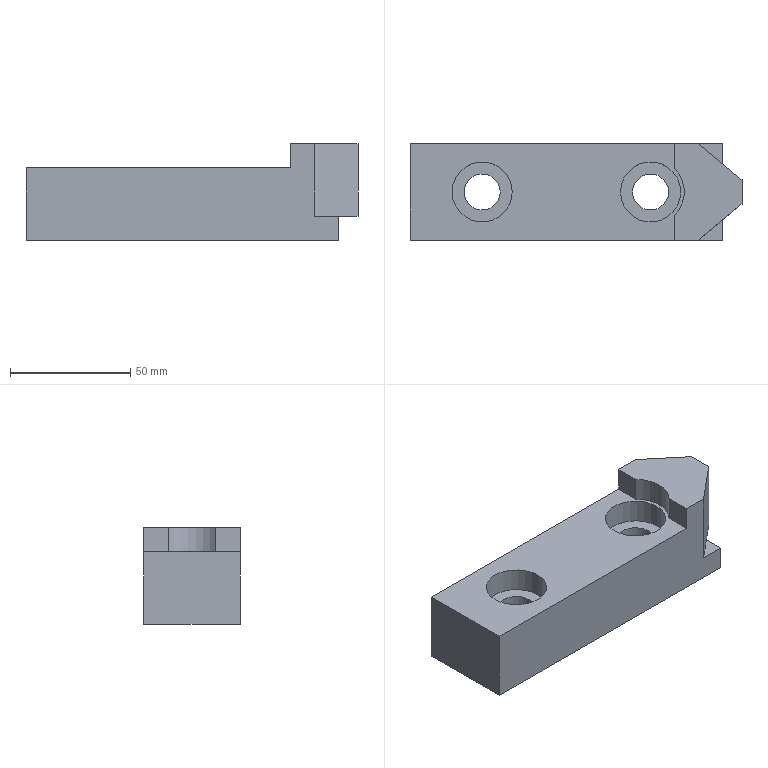Part | SolidWorks | features ICE 5, Extrusion 1 | 1 solid | 26 faces | box 138 x 40 x 40 mm | volume 148074 mm3 | plane 17 | cylinder 9 | commonest cylinder face diameters 15 x4 25 x4 28 x1
STEP:
#1=CARTESIAN_POINT('',(-47.5,0.,20.));
#2=VERTEX_POINT('',#1);
#3=CARTESIAN_POINT('',(-22.5,0.,20.));
#4=VERTEX_POINT('',#3);
#5=CARTESIAN_POINT('',(-35.,0.,20.));
#6=DIRECTION('',(0.,0.,1.));
#7=DIRECTION('',(1.,0.,0.));
#8=AXIS2_PLACEMENT_3D('',#5,#6,#7);
#9=CIRCLE('',#8,12.5);
#10=EDGE_CURVE('',#2,#4,#9,.T.);
#11=ORIENTED_EDGE('',*,*,#10,.F.);
#12=CARTESIAN_POINT('',(-47.5,0.,30.));
#13=VERTEX_POINT('',#12);
#14=CARTESIAN_POINT('',(-47.5,0.,20.));
#15=DIRECTION('',(0.,0.,1.));
#16=VECTOR('',#15,1000.);
#17=LINE('',#14,#16);
#18=EDGE_CURVE('',#2,#13,#17,.T.);
#19=ORIENTED_EDGE('',*,*,#18,.T.);
#20=CARTESIAN_POINT('',(-22.5,0.,30.));
#21=VERTEX_POINT('',#20);
#22=CARTESIAN_POINT('',(-35.,0.,30.));
#23=DIRECTION('',(0.,0.,1.));
#24=DIRECTION('',(1.,0.,0.));
#25=AXIS2_PLACEMENT_3D('',#22,#23,#24);
#26=CIRCLE('',#25,12.5);
#27=EDGE_CURVE('',#13,#21,#26,.T.);
#28=ORIENTED_EDGE('',*,*,#27,.T.);
#29=CARTESIAN_POINT('',(-22.5,0.,20.));
#30=DIRECTION('',(0.,0.,1.));
#31=VECTOR('',#30,1000.);
#32=LINE('',#29,#31);
#33=EDGE_CURVE('',#4,#21,#32,.T.);
#34=ORIENTED_EDGE('',*,*,#33,.F.);
#35=EDGE_LOOP('',(#11,#19,#28,#34));
#36=FACE_OUTER_BOUND('',#35,.T.);
#37=CARTESIAN_POINT('',(-35.,0.,20.));
#38=DIRECTION('',(0.,0.,1.));
#39=DIRECTION('',(1.,0.,0.));
#40=AXIS2_PLACEMENT_3D('',#37,#38,#39);
#41=CYLINDRICAL_SURFACE('',#40,12.5);
#42=ADVANCED_FACE('',(#36),#41,.F.);
#43=CARTESIAN_POINT('',(22.5,0.,20.));
#44=VERTEX_POINT('',#43);
#45=CARTESIAN_POINT('',(47.5,0.,20.));
#46=VERTEX_POINT('',#45);
#47=CARTESIAN_POINT('',(35.,0.,20.));
#48=DIRECTION('',(0.,0.,1.));
#49=DIRECTION('',(1.,0.,0.));
#50=AXIS2_PLACEMENT_3D('',#47,#48,#49);
#51=CIRCLE('',#50,12.5);
#52=EDGE_CURVE('',#44,#46,#51,.T.);
#53=ORIENTED_EDGE('',*,*,#52,.F.);
#54=CARTESIAN_POINT('',(22.5,0.,30.));
#55=VERTEX_POINT('',#54);
#56=CARTESIAN_POINT('',(22.5,0.,20.));
#57=DIRECTION('',(0.,0.,1.));
#58=VECTOR('',#57,1000.);
#59=LINE('',#56,#58);
#60=EDGE_CURVE('',#44,#55,#59,.T.);
#61=ORIENTED_EDGE('',*,*,#60,.T.);
#62=CARTESIAN_POINT('',(47.5,0.,30.));
#63=VERTEX_POINT('',#62);
#64=CARTESIAN_POINT('',(35.,0.,30.));
#65=DIRECTION('',(0.,0.,1.));
#66=DIRECTION('',(1.,0.,0.));
#67=AXIS2_PLACEMENT_3D('',#64,#65,#66);
#68=CIRCLE('',#67,12.5);
#69=EDGE_CURVE('',#55,#63,#68,.T.);
#70=ORIENTED_EDGE('',*,*,#69,.T.);
#71=CARTESIAN_POINT('',(47.5,0.,20.));
#72=DIRECTION('',(0.,0.,1.));
#73=VECTOR('',#72,1000.);
#74=LINE('',#71,#73);
#75=EDGE_CURVE('',#46,#63,#74,.T.);
#76=ORIENTED_EDGE('',*,*,#75,.F.);
#77=EDGE_LOOP('',(#53,#61,#70,#76));
#78=FACE_OUTER_BOUND('',#77,.T.);
#79=CARTESIAN_POINT('',(35.,0.,20.));
#80=DIRECTION('',(0.,0.,1.));
#81=DIRECTION('',(1.,0.,0.));
#82=AXIS2_PLACEMENT_3D('',#79,#80,#81);
#83=CYLINDRICAL_SURFACE('',#82,12.5);
#84=ADVANCED_FACE('',(#78),#83,.F.);
#85=CARTESIAN_POINT('',(42.5,0.,20.));
#86=VERTEX_POINT('',#85);
#87=CARTESIAN_POINT('',(27.5,0.,20.));
#88=VERTEX_POINT('',#87);
#89=CARTESIAN_POINT('',(35.,0.,20.));
#90=DIRECTION('',(0.,0.,-1.));
#91=DIRECTION('',(1.,0.,0.));
#92=AXIS2_PLACEMENT_3D('',#89,#90,#91);
#93=CIRCLE('',#92,7.5);
#94=EDGE_CURVE('',#86,#88,#93,.T.);
#95=ORIENTED_EDGE('',*,*,#94,.F.);
#96=CARTESIAN_POINT('',(42.5,0.,0.));
#97=VERTEX_POINT('',#96);
#98=CARTESIAN_POINT('',(42.5,0.,40.));
#99=DIRECTION('',(0.,0.,-1.));
#100=VECTOR('',#99,1000.);
#101=LINE('',#98,#100);
#102=EDGE_CURVE('',#86,#97,#101,.T.);
#103=ORIENTED_EDGE('',*,*,#102,.T.);
#104=CARTESIAN_POINT('',(27.5,0.,0.));
#105=VERTEX_POINT('',#104);
#106=CARTESIAN_POINT('',(35.,0.,0.));
#107=DIRECTION('',(0.,0.,-1.));
#108=DIRECTION('',(-1.,0.,0.));
#109=AXIS2_PLACEMENT_3D('',#106,#107,#108);
#110=CIRCLE('',#109,7.5);
#111=EDGE_CURVE('',#97,#105,#110,.T.);
#112=ORIENTED_EDGE('',*,*,#111,.T.);
#113=CARTESIAN_POINT('',(27.5,0.,40.));
#114=DIRECTION('',(0.,0.,-1.));
#115=VECTOR('',#114,1000.);
#116=LINE('',#113,#115);
#117=EDGE_CURVE('',#88,#105,#116,.T.);
#118=ORIENTED_EDGE('',*,*,#117,.F.);
#119=EDGE_LOOP('',(#95,#103,#112,#118));
#120=FACE_OUTER_BOUND('',#119,.T.);
#121=CARTESIAN_POINT('',(35.,0.,40.));
#122=DIRECTION('',(0.,0.,-1.));
#123=DIRECTION('',(-1.,0.,0.));
#124=AXIS2_PLACEMENT_3D('',#121,#122,#123);
#125=CYLINDRICAL_SURFACE('',#124,7.5);
#126=ADVANCED_FACE('',(#120),#125,.F.);
#127=CARTESIAN_POINT('',(-27.5,0.,20.));
#128=VERTEX_POINT('',#127);
#129=CARTESIAN_POINT('',(-42.5,0.,20.));
#130=VERTEX_POINT('',#129);
#131=CARTESIAN_POINT('',(-35.,0.,20.));
#132=DIRECTION('',(0.,0.,-1.));
#133=DIRECTION('',(1.,0.,0.));
#134=AXIS2_PLACEMENT_3D('',#131,#132,#133);
#135=CIRCLE('',#134,7.5);
#136=EDGE_CURVE('',#128,#130,#135,.T.);
#137=ORIENTED_EDGE('',*,*,#136,.F.);
#138=CARTESIAN_POINT('',(-27.5,0.,0.));
#139=VERTEX_POINT('',#138);
#140=CARTESIAN_POINT('',(-27.5,0.,40.));
#141=DIRECTION('',(0.,0.,-1.));
#142=VECTOR('',#141,1000.);
#143=LINE('',#140,#142);
#144=EDGE_CURVE('',#128,#139,#143,.T.);
#145=ORIENTED_EDGE('',*,*,#144,.T.);
#146=CARTESIAN_POINT('',(-42.5,0.,0.));
#147=VERTEX_POINT('',#146);
#148=CARTESIAN_POINT('',(-35.,0.,0.));
#149=DIRECTION('',(0.,0.,-1.));
#150=DIRECTION('',(-1.,0.,0.));
#151=AXIS2_PLACEMENT_3D('',#148,#149,#150);
#152=CIRCLE('',#151,7.5);
#153=EDGE_CURVE('',#139,#147,#152,.T.);
#154=ORIENTED_EDGE('',*,*,#153,.T.);
#155=CARTESIAN_POINT('',(-42.5,0.,40.));
#156=DIRECTION('',(0.,0.,-1.));
#157=VECTOR('',#156,1000.);
#158=LINE('',#155,#157);
#159=EDGE_CURVE('',#130,#147,#158,.T.);
#160=ORIENTED_EDGE('',*,*,#159,.F.);
#161=EDGE_LOOP('',(#137,#145,#154,#160));
#162=FACE_OUTER_BOUND('',#161,.T.);
#163=CARTESIAN_POINT('',(-35.,0.,40.));
#164=DIRECTION('',(0.,0.,-1.));
#165=DIRECTION('',(-1.,0.,0.));
#166=AXIS2_PLACEMENT_3D('',#163,#164,#165);
#167=CYLINDRICAL_SURFACE('',#166,7.5);
#168=ADVANCED_FACE('',(#162),#167,.F.);
#169=ORIENTED_EDGE('',*,*,#144,.F.);
#170=CARTESIAN_POINT('',(-35.,0.,20.));
#171=DIRECTION('',(0.,0.,-1.));
#172=DIRECTION('',(1.,0.,0.));
#173=AXIS2_PLACEMENT_3D('',#170,#171,#172);
#174=CIRCLE('',#173,7.5);
#175=EDGE_CURVE('',#130,#128,#174,.T.);
#176=ORIENTED_EDGE('',*,*,#175,.F.);
#177=ORIENTED_EDGE('',*,*,#159,.T.);
#178=CARTESIAN_POINT('',(-35.,0.,0.));
#179=DIRECTION('',(0.,0.,-1.));
#180=DIRECTION('',(-1.,0.,0.));
#181=AXIS2_PLACEMENT_3D('',#178,#179,#180);
#182=CIRCLE('',#181,7.5);
#183=EDGE_CURVE('',#147,#139,#182,.T.);
#184=ORIENTED_EDGE('',*,*,#183,.T.);
#185=EDGE_LOOP('',(#169,#176,#177,#184));
#186=FACE_OUTER_BOUND('',#185,.T.);
#187=CARTESIAN_POINT('',(-35.,0.,40.));
#188=DIRECTION('',(0.,0.,-1.));
#189=DIRECTION('',(-1.,0.,0.));
#190=AXIS2_PLACEMENT_3D('',#187,#188,#189);
#191=CYLINDRICAL_SURFACE('',#190,7.5);
#192=ADVANCED_FACE('',(#186),#191,.F.);
#193=ORIENTED_EDGE('',*,*,#102,.F.);
#194=CARTESIAN_POINT('',(35.,0.,20.));
#195=DIRECTION('',(0.,0.,-1.));
#196=DIRECTION('',(1.,0.,0.));
#197=AXIS2_PLACEMENT_3D('',#194,#195,#196);
#198=CIRCLE('',#197,7.5);
#199=EDGE_CURVE('',#88,#86,#198,.T.);
#200=ORIENTED_EDGE('',*,*,#199,.F.);
#201=ORIENTED_EDGE('',*,*,#117,.T.);
#202=CARTESIAN_POINT('',(35.,0.,0.));
#203=DIRECTION('',(0.,0.,-1.));
#204=DIRECTION('',(-1.,0.,0.));
#205=AXIS2_PLACEMENT_3D('',#202,#203,#204);
#206=CIRCLE('',#205,7.5);
#207=EDGE_CURVE('',#105,#97,#206,.T.);
#208=ORIENTED_EDGE('',*,*,#207,.T.);
#209=EDGE_LOOP('',(#193,#200,#201,#208));
#210=FACE_OUTER_BOUND('',#209,.T.);
#211=CARTESIAN_POINT('',(35.,0.,40.));
#212=DIRECTION('',(0.,0.,-1.));
#213=DIRECTION('',(-1.,0.,0.));
#214=AXIS2_PLACEMENT_3D('',#211,#212,#213);
#215=CYLINDRICAL_SURFACE('',#214,7.5);
#216=ADVANCED_FACE('',(#210),#215,.F.);
#217=CARTESIAN_POINT('',(45.,-9.798,30.));
#218=VERTEX_POINT('',#217);
#219=CARTESIAN_POINT('',(45.,-9.798,40.));
#220=VERTEX_POINT('',#219);
#221=CARTESIAN_POINT('',(45.,-9.798,70.));
#222=DIRECTION('',(0.,0.,1.));
#223=VECTOR('',#222,1000.);
#224=LINE('',#221,#223);
#225=EDGE_CURVE('',#218,#220,#224,.T.);
#226=ORIENTED_EDGE('',*,*,#225,.F.);
#227=CARTESIAN_POINT('',(45.,-20.,30.));
#228=VERTEX_POINT('',#227);
#229=CARTESIAN_POINT('',(45.,20.,30.));
#230=DIRECTION('',(0.,-1.,0.));
#231=VECTOR('',#230,1000.);
#232=LINE('',#229,#231);
#233=EDGE_CURVE('',#218,#228,#232,.T.);
#234=ORIENTED_EDGE('',*,*,#233,.T.);
#235=CARTESIAN_POINT('',(45.,-20.,40.));
#236=VERTEX_POINT('',#235);
#237=CARTESIAN_POINT('',(45.,-20.,30.));
#238=DIRECTION('',(0.,0.,1.));
#239=VECTOR('',#238,1000.);
#240=LINE('',#237,#239);
#241=EDGE_CURVE('',#228,#236,#240,.T.);
#242=ORIENTED_EDGE('',*,*,#241,.T.);
#243=CARTESIAN_POINT('',(45.,20.,40.));
#244=DIRECTION('',(0.,-1.,0.));
#245=VECTOR('',#244,1000.);
#246=LINE('',#243,#245);
#247=EDGE_CURVE('',#220,#236,#246,.T.);
#248=ORIENTED_EDGE('',*,*,#247,.F.);
#249=EDGE_LOOP('',(#226,#234,#242,#248));
#250=FACE_OUTER_BOUND('',#249,.T.);
#251=CARTESIAN_POINT('',(45.,20.,30.));
#252=DIRECTION('',(1.,0.,0.));
#253=DIRECTION('',(0.,0.,-1.));
#254=AXIS2_PLACEMENT_3D('',#251,#252,#253);
#255=PLANE('',#254);
#256=ADVANCED_FACE('',(#250),#255,.F.);
#257=CARTESIAN_POINT('',(45.,9.798,40.));
#258=VERTEX_POINT('',#257);
#259=CARTESIAN_POINT('',(45.,9.798,30.));
#260=VERTEX_POINT('',#259);
#261=CARTESIAN_POINT('',(45.,9.798,70.));
#262=DIRECTION('',(0.,0.,-1.));
#263=VECTOR('',#262,1000.);
#264=LINE('',#261,#263);
#265=EDGE_CURVE('',#258,#260,#264,.T.);
#266=ORIENTED_EDGE('',*,*,#265,.F.);
#267=CARTESIAN_POINT('',(45.,20.,40.));
#268=VERTEX_POINT('',#267);
#269=CARTESIAN_POINT('',(45.,20.,40.));
#270=DIRECTION('',(0.,-1.,0.));
#271=VECTOR('',#270,1000.);
#272=LINE('',#269,#271);
#273=EDGE_CURVE('',#268,#258,#272,.T.);
#274=ORIENTED_EDGE('',*,*,#273,.F.);
#275=CARTESIAN_POINT('',(45.,20.,30.));
#276=VERTEX_POINT('',#275);
#277=CARTESIAN_POINT('',(45.,20.,30.));
#278=DIRECTION('',(0.,0.,1.));
#279=VECTOR('',#278,1000.);
#280=LINE('',#277,#279);
#281=EDGE_CURVE('',#276,#268,#280,.T.);
#282=ORIENTED_EDGE('',*,*,#281,.F.);
#283=CARTESIAN_POINT('',(45.,20.,30.));
#284=DIRECTION('',(0.,-1.,0.));
#285=VECTOR('',#284,1000.);
#286=LINE('',#283,#285);
#287=EDGE_CURVE('',#276,#260,#286,.T.);
#288=ORIENTED_EDGE('',*,*,#287,.T.);
#289=EDGE_LOOP('',(#266,#274,#282,#288));
#290=FACE_OUTER_BOUND('',#289,.T.);
#291=CARTESIAN_POINT('',(45.,20.,30.));
#292=DIRECTION('',(1.,0.,0.));
#293=DIRECTION('',(0.,0.,-1.));
#294=AXIS2_PLACEMENT_3D('',#291,#292,#293);
#295=PLANE('',#294);
#296=ADVANCED_FACE('',(#290),#295,.F.);
#297=CARTESIAN_POINT('',(65.,11.667,10.));
#298=VERTEX_POINT('',#297);
#299=CARTESIAN_POINT('',(55.,20.,10.));
#300=VERTEX_POINT('',#299);
#301=CARTESIAN_POINT('',(55.,20.,10.));
#302=DIRECTION('',(-0.7682,0.6402,0.));
#303=VECTOR('',#302,1000.);
#304=LINE('',#301,#303);
#305=EDGE_CURVE('',#298,#300,#304,.T.);
#306=ORIENTED_EDGE('',*,*,#305,.F.);
#307=CARTESIAN_POINT('',(65.,20.,10.));
#308=VERTEX_POINT('',#307);
#309=CARTESIAN_POINT('',(65.,20.,10.));
#310=DIRECTION('',(0.,1.,0.));
#311=VECTOR('',#310,1000.);
#312=LINE('',#309,#311);
#313=EDGE_CURVE('',#298,#308,#312,.T.);
#314=ORIENTED_EDGE('',*,*,#313,.T.);
#315=CARTESIAN_POINT('',(-65.,20.,10.));
#316=DIRECTION('',(-1.,0.,0.));
#317=VECTOR('',#316,1000.);
#318=LINE('',#315,#317);
#319=EDGE_CURVE('',#308,#300,#318,.T.);
#320=ORIENTED_EDGE('',*,*,#319,.T.);
#321=EDGE_LOOP('',(#306,#314,#320));
#322=FACE_OUTER_BOUND('',#321,.T.);
#323=CARTESIAN_POINT('',(0.,0.,10.));
#324=DIRECTION('',(0.,0.,1.));
#325=DIRECTION('',(1.,0.,0.));
#326=AXIS2_PLACEMENT_3D('',#323,#324,#325);
#327=PLANE('',#326);
#328=ADVANCED_FACE('',(#322),#327,.T.);
#329=CARTESIAN_POINT('',(65.,-20.,0.));
#330=VERTEX_POINT('',#329);
#331=CARTESIAN_POINT('',(65.,20.,0.));
#332=VERTEX_POINT('',#331);
#333=CARTESIAN_POINT('',(65.,20.,0.));
#334=DIRECTION('',(0.,1.,0.));
#335=VECTOR('',#334,1000.);
#336=LINE('',#333,#335);
#337=EDGE_CURVE('',#330,#332,#336,.T.);
#338=ORIENTED_EDGE('',*,*,#337,.T.);
#339=CARTESIAN_POINT('',(65.,20.,10.));
#340=DIRECTION('',(0.,0.,-1.));
#341=VECTOR('',#340,1000.);
#342=LINE('',#339,#341);
#343=EDGE_CURVE('',#308,#332,#342,.T.);
#344=ORIENTED_EDGE('',*,*,#343,.F.);
#345=ORIENTED_EDGE('',*,*,#313,.F.);
#346=CARTESIAN_POINT('',(65.,-11.667,10.));
#347=VERTEX_POINT('',#346);
#348=CARTESIAN_POINT('',(65.,20.,10.));
#349=DIRECTION('',(0.,1.,0.));
#350=VECTOR('',#349,1000.);
#351=LINE('',#348,#350);
#352=EDGE_CURVE('',#347,#298,#351,.T.);
#353=ORIENTED_EDGE('',*,*,#352,.F.);
#354=CARTESIAN_POINT('',(65.,-20.,10.));
#355=VERTEX_POINT('',#354);
#356=CARTESIAN_POINT('',(65.,20.,10.));
#357=DIRECTION('',(0.,1.,0.));
#358=VECTOR('',#357,1000.);
#359=LINE('',#356,#358);
#360=EDGE_CURVE('',#355,#347,#359,.T.);
#361=ORIENTED_EDGE('',*,*,#360,.F.);
#362=CARTESIAN_POINT('',(65.,-20.,10.));
#363=DIRECTION('',(0.,0.,-1.));
#364=VECTOR('',#363,1000.);
#365=LINE('',#362,#364);
#366=EDGE_CURVE('',#355,#330,#365,.T.);
#367=ORIENTED_EDGE('',*,*,#366,.T.);
#368=EDGE_LOOP('',(#338,#344,#345,#353,#361,#367));
#369=FACE_OUTER_BOUND('',#368,.T.);
#370=CARTESIAN_POINT('',(65.,20.,10.));
#371=DIRECTION('',(-1.,0.,0.));
#372=DIRECTION('',(0.,0.,1.));
#373=AXIS2_PLACEMENT_3D('',#370,#371,#372);
#374=PLANE('',#373);
#375=ADVANCED_FACE('',(#369),#374,.F.);
#376=CARTESIAN_POINT('',(-65.,20.,30.));
#377=VERTEX_POINT('',#376);
#378=CARTESIAN_POINT('',(-65.,20.,30.));
#379=DIRECTION('',(1.,0.,0.));
#380=VECTOR('',#379,1000.);
#381=LINE('',#378,#380);
#382=EDGE_CURVE('',#377,#276,#381,.T.);
#383=ORIENTED_EDGE('',*,*,#382,.T.);
#384=ORIENTED_EDGE('',*,*,#281,.T.);
#385=CARTESIAN_POINT('',(55.,20.,40.));
#386=VERTEX_POINT('',#385);
#387=CARTESIAN_POINT('',(-65.,20.,40.));
#388=DIRECTION('',(-1.,0.,0.));
#389=VECTOR('',#388,1000.);
#390=LINE('',#387,#389);
#391=EDGE_CURVE('',#386,#268,#390,.T.);
#392=ORIENTED_EDGE('',*,*,#391,.F.);
#393=CARTESIAN_POINT('',(55.,20.,40.));
#394=DIRECTION('',(0.,0.,-1.));
#395=VECTOR('',#394,1000.);
#396=LINE('',#393,#395);
#397=EDGE_CURVE('',#386,#300,#396,.T.);
#398=ORIENTED_EDGE('',*,*,#397,.T.);
#399=ORIENTED_EDGE('',*,*,#319,.F.);
#400=ORIENTED_EDGE('',*,*,#343,.T.);
#401=CARTESIAN_POINT('',(-65.,20.,0.));
#402=VERTEX_POINT('',#401);
#403=CARTESIAN_POINT('',(-65.,20.,0.));
#404=DIRECTION('',(-1.,0.,0.));
#405=VECTOR('',#404,1000.);
#406=LINE('',#403,#405);
#407=EDGE_CURVE('',#332,#402,#406,.T.);
#408=ORIENTED_EDGE('',*,*,#407,.T.);
#409=CARTESIAN_POINT('',(-65.,20.,10.));
#410=DIRECTION('',(0.,0.,-1.));
#411=VECTOR('',#410,1000.);
#412=LINE('',#409,#411);
#413=EDGE_CURVE('',#377,#402,#412,.T.);
#414=ORIENTED_EDGE('',*,*,#413,.F.);
#415=EDGE_LOOP('',(#383,#384,#392,#398,#399,#400,#408,#414));
#416=FACE_OUTER_BOUND('',#415,.T.);
#417=CARTESIAN_POINT('',(-65.,20.,10.));
#418=DIRECTION('',(0.,-1.,0.));
#419=DIRECTION('',(0.,0.,-1.));
#420=AXIS2_PLACEMENT_3D('',#417,#418,#419);
#421=PLANE('',#420);
#422=ADVANCED_FACE('',(#416),#421,.F.);
#423=CARTESIAN_POINT('',(-65.,-20.,30.));
#424=VERTEX_POINT('',#423);
#425=CARTESIAN_POINT('',(-65.,-20.,0.));
#426=VERTEX_POINT('',#425);
#427=CARTESIAN_POINT('',(-65.,-20.,10.));
#428=DIRECTION('',(0.,0.,-1.));
#429=VECTOR('',#428,1000.);
#430=LINE('',#427,#429);
#431=EDGE_CURVE('',#424,#426,#430,.T.);
#432=ORIENTED_EDGE('',*,*,#431,.F.);
#433=CARTESIAN_POINT('',(-65.,20.,30.));
#434=DIRECTION('',(0.,-1.,0.));
#435=VECTOR('',#434,1000.);
#436=LINE('',#433,#435);
#437=EDGE_CURVE('',#377,#424,#436,.T.);
#438=ORIENTED_EDGE('',*,*,#437,.F.);
#439=ORIENTED_EDGE('',*,*,#413,.T.);
#440=CARTESIAN_POINT('',(-65.,20.,0.));
#441=DIRECTION('',(0.,-1.,0.));
#442=VECTOR('',#441,1000.);
#443=LINE('',#440,#442);
#444=EDGE_CURVE('',#402,#426,#443,.T.);
#445=ORIENTED_EDGE('',*,*,#444,.T.);
#446=EDGE_LOOP('',(#432,#438,#439,#445));
#447=FACE_OUTER_BOUND('',#446,.T.);
#448=CARTESIAN_POINT('',(-65.,20.,10.));
#449=DIRECTION('',(1.,0.,0.));
#450=DIRECTION('',(0.,0.,-1.));
#451=AXIS2_PLACEMENT_3D('',#448,#449,#450);
#452=PLANE('',#451);
#453=ADVANCED_FACE('',(#447),#452,.F.);
#454=CARTESIAN_POINT('',(55.,-20.,40.));
#455=VERTEX_POINT('',#454);
#456=CARTESIAN_POINT('',(-65.,-20.,40.));
#457=DIRECTION('',(1.,0.,0.));
#458=VECTOR('',#457,1000.);
#459=LINE('',#456,#458);
#460=EDGE_CURVE('',#236,#455,#459,.T.);
#461=ORIENTED_EDGE('',*,*,#460,.F.);
#462=ORIENTED_EDGE('',*,*,#241,.F.);
#463=CARTESIAN_POINT('',(-65.,-20.,30.));
#464=DIRECTION('',(1.,0.,0.));
#465=VECTOR('',#464,1000.);
#466=LINE('',#463,#465);
#467=EDGE_CURVE('',#424,#228,#466,.T.);
#468=ORIENTED_EDGE('',*,*,#467,.F.);
#469=ORIENTED_EDGE('',*,*,#431,.T.);
#470=CARTESIAN_POINT('',(-65.,-20.,0.));
#471=DIRECTION('',(1.,0.,0.));
#472=VECTOR('',#471,1000.);
#473=LINE('',#470,#472);
#474=EDGE_CURVE('',#426,#330,#473,.T.);
#475=ORIENTED_EDGE('',*,*,#474,.T.);
#476=ORIENTED_EDGE('',*,*,#366,.F.);
#477=CARTESIAN_POINT('',(55.,-20.,10.));
#478=VERTEX_POINT('',#477);
#479=CARTESIAN_POINT('',(-65.,-20.,10.));
#480=DIRECTION('',(1.,0.,0.));
#481=VECTOR('',#480,1000.);
#482=LINE('',#479,#481);
#483=EDGE_CURVE('',#478,#355,#482,.T.);
#484=ORIENTED_EDGE('',*,*,#483,.F.);
#485=CARTESIAN_POINT('',(55.,-20.,40.));
#486=DIRECTION('',(0.,0.,-1.));
#487=VECTOR('',#486,1000.);
#488=LINE('',#485,#487);
#489=EDGE_CURVE('',#455,#478,#488,.T.);
#490=ORIENTED_EDGE('',*,*,#489,.F.);
#491=EDGE_LOOP('',(#461,#462,#468,#469,#475,#476,#484,#490));
#492=FACE_OUTER_BOUND('',#491,.T.);
#493=CARTESIAN_POINT('',(-65.,-20.,10.));
#494=DIRECTION('',(0.,1.,0.));
#495=DIRECTION('',(0.,0.,1.));
#496=AXIS2_PLACEMENT_3D('',#493,#494,#495);
#497=PLANE('',#496);
#498=ADVANCED_FACE('',(#492),#497,.F.);
#499=CARTESIAN_POINT('',(55.,-20.,10.));
#500=DIRECTION('',(0.7682,0.6402,0.));
#501=VECTOR('',#500,1000.);
#502=LINE('',#499,#501);
#503=EDGE_CURVE('',#478,#347,#502,.T.);
#504=ORIENTED_EDGE('',*,*,#503,.F.);
#505=ORIENTED_EDGE('',*,*,#483,.T.);
#506=ORIENTED_EDGE('',*,*,#360,.T.);
#507=EDGE_LOOP('',(#504,#505,#506));
#508=FACE_OUTER_BOUND('',#507,.T.);
#509=CARTESIAN_POINT('',(0.,0.,10.));
#510=DIRECTION('',(0.,0.,1.));
#511=DIRECTION('',(1.,0.,0.));
#512=AXIS2_PLACEMENT_3D('',#509,#510,#511);
#513=PLANE('',#512);
#514=ADVANCED_FACE('',(#508),#513,.T.);
#515=ORIENTED_EDGE('',*,*,#207,.F.);
#516=ORIENTED_EDGE('',*,*,#111,.F.);
#517=EDGE_LOOP('',(#515,#516));
#518=FACE_BOUND('',#517,.T.);
#519=ORIENTED_EDGE('',*,*,#183,.F.);
#520=ORIENTED_EDGE('',*,*,#153,.F.);
#521=EDGE_LOOP('',(#519,#520));
#522=FACE_BOUND('',#521,.T.);
#523=ORIENTED_EDGE('',*,*,#337,.F.);
#524=ORIENTED_EDGE('',*,*,#474,.F.);
#525=ORIENTED_EDGE('',*,*,#444,.F.);
#526=ORIENTED_EDGE('',*,*,#407,.F.);
#527=EDGE_LOOP('',(#523,#524,#525,#526));
#528=FACE_OUTER_BOUND('',#527,.T.);
#529=CARTESIAN_POINT('',(0.,0.,0.));
#530=DIRECTION('',(0.,0.,1.));
#531=DIRECTION('',(1.,0.,0.));
#532=AXIS2_PLACEMENT_3D('',#529,#530,#531);
#533=PLANE('',#532);
#534=ADVANCED_FACE('',(#518,#522,#528),#533,.F.);
#535=CARTESIAN_POINT('',(73.,-5.,10.));
#536=VERTEX_POINT('',#535);
#537=CARTESIAN_POINT('',(55.,-20.,10.));
#538=DIRECTION('',(0.7682,0.6402,0.));
#539=VECTOR('',#538,1000.);
#540=LINE('',#537,#539);
#541=EDGE_CURVE('',#347,#536,#540,.T.);
#542=ORIENTED_EDGE('',*,*,#541,.F.);
#543=ORIENTED_EDGE('',*,*,#352,.T.);
#544=CARTESIAN_POINT('',(73.,5.,10.));
#545=VERTEX_POINT('',#544);
#546=CARTESIAN_POINT('',(55.,20.,10.));
#547=DIRECTION('',(-0.7682,0.6402,0.));
#548=VECTOR('',#547,1000.);
#549=LINE('',#546,#548);
#550=EDGE_CURVE('',#545,#298,#549,.T.);
#551=ORIENTED_EDGE('',*,*,#550,.F.);
#552=CARTESIAN_POINT('',(73.,5.,10.));
#553=DIRECTION('',(0.,1.,0.));
#554=VECTOR('',#553,1000.);
#555=LINE('',#552,#554);
#556=EDGE_CURVE('',#536,#545,#555,.T.);
#557=ORIENTED_EDGE('',*,*,#556,.F.);
#558=EDGE_LOOP('',(#542,#543,#551,#557));
#559=FACE_OUTER_BOUND('',#558,.T.);
#560=CARTESIAN_POINT('',(0.,0.,10.));
#561=DIRECTION('',(0.,0.,1.));
#562=DIRECTION('',(1.,0.,0.));
#563=AXIS2_PLACEMENT_3D('',#560,#561,#562);
#564=PLANE('',#563);
#565=ADVANCED_FACE('',(#559),#564,.F.);
#566=ORIENTED_EDGE('',*,*,#503,.T.);
#567=ORIENTED_EDGE('',*,*,#541,.T.);
#568=CARTESIAN_POINT('',(73.,-5.,40.));
#569=VERTEX_POINT('',#568);
#570=CARTESIAN_POINT('',(73.,-5.,40.));
#571=DIRECTION('',(0.,0.,-1.));
#572=VECTOR('',#571,1000.);
#573=LINE('',#570,#572);
#574=EDGE_CURVE('',#569,#536,#573,.T.);
#575=ORIENTED_EDGE('',*,*,#574,.F.);
#576=CARTESIAN_POINT('',(55.,-20.,40.));
#577=DIRECTION('',(0.7682,0.6402,0.));
#578=VECTOR('',#577,1000.);
#579=LINE('',#576,#578);
#580=EDGE_CURVE('',#455,#569,#579,.T.);
#581=ORIENTED_EDGE('',*,*,#580,.F.);
#582=ORIENTED_EDGE('',*,*,#489,.T.);
#583=EDGE_LOOP('',(#566,#567,#575,#581,#582));
#584=FACE_OUTER_BOUND('',#583,.T.);
#585=CARTESIAN_POINT('',(55.,-20.,40.));
#586=DIRECTION('',(-0.6402,0.7682,0.));
#587=DIRECTION('',(-0.7682,-0.6402,0.));
#588=AXIS2_PLACEMENT_3D('',#585,#586,#587);
#589=PLANE('',#588);
#590=ADVANCED_FACE('',(#584),#589,.F.);
#591=ORIENTED_EDGE('',*,*,#556,.T.);
#592=CARTESIAN_POINT('',(73.,5.,40.));
#593=VERTEX_POINT('',#592);
#594=CARTESIAN_POINT('',(73.,5.,40.));
#595=DIRECTION('',(0.,0.,-1.));
#596=VECTOR('',#595,1000.);
#597=LINE('',#594,#596);
#598=EDGE_CURVE('',#593,#545,#597,.T.);
#599=ORIENTED_EDGE('',*,*,#598,.F.);
#600=CARTESIAN_POINT('',(73.,5.,40.));
#601=DIRECTION('',(0.,1.,0.));
#602=VECTOR('',#601,1000.);
#603=LINE('',#600,#602);
#604=EDGE_CURVE('',#569,#593,#603,.T.);
#605=ORIENTED_EDGE('',*,*,#604,.F.);
#606=ORIENTED_EDGE('',*,*,#574,.T.);
#607=EDGE_LOOP('',(#591,#599,#605,#606));
#608=FACE_OUTER_BOUND('',#607,.T.);
#609=CARTESIAN_POINT('',(73.,5.,40.));
#610=DIRECTION('',(-1.,0.,0.));
#611=DIRECTION('',(0.,0.,1.));
#612=AXIS2_PLACEMENT_3D('',#609,#610,#611);
#613=PLANE('',#612);
#614=ADVANCED_FACE('',(#608),#613,.F.);
#615=ORIENTED_EDGE('',*,*,#550,.T.);
#616=ORIENTED_EDGE('',*,*,#305,.T.);
#617=ORIENTED_EDGE('',*,*,#397,.F.);
#618=CARTESIAN_POINT('',(55.,20.,40.));
#619=DIRECTION('',(-0.7682,0.6402,0.));
#620=VECTOR('',#619,1000.);
#621=LINE('',#618,#620);
#622=EDGE_CURVE('',#593,#386,#621,.T.);
#623=ORIENTED_EDGE('',*,*,#622,.F.);
#624=ORIENTED_EDGE('',*,*,#598,.T.);
#625=EDGE_LOOP('',(#615,#616,#617,#623,#624));
#626=FACE_OUTER_BOUND('',#625,.T.);
#627=CARTESIAN_POINT('',(55.,20.,40.));
#628=DIRECTION('',(-0.6402,-0.7682,0.));
#629=DIRECTION('',(0.7682,-0.6402,0.));
#630=AXIS2_PLACEMENT_3D('',#627,#628,#629);
#631=PLANE('',#630);
#632=ADVANCED_FACE('',(#626),#631,.F.);
#633=ORIENTED_EDGE('',*,*,#273,.T.);
#634=CARTESIAN_POINT('',(35.,0.,40.));
#635=DIRECTION('',(0.,0.,-1.));
#636=DIRECTION('',(1.,0.,0.));
#637=AXIS2_PLACEMENT_3D('',#634,#635,#636);
#638=CIRCLE('',#637,14.);
#639=EDGE_CURVE('',#258,#220,#638,.T.);
#640=ORIENTED_EDGE('',*,*,#639,.T.);
#641=ORIENTED_EDGE('',*,*,#247,.T.);
#642=ORIENTED_EDGE('',*,*,#460,.T.);
#643=ORIENTED_EDGE('',*,*,#580,.T.);
#644=ORIENTED_EDGE('',*,*,#604,.T.);
#645=ORIENTED_EDGE('',*,*,#622,.T.);
#646=ORIENTED_EDGE('',*,*,#391,.T.);
#647=EDGE_LOOP('',(#633,#640,#641,#642,#643,#644,#645,#646));
#648=FACE_OUTER_BOUND('',#647,.T.);
#649=CARTESIAN_POINT('',(0.,0.,40.));
#650=DIRECTION('',(0.,0.,1.));
#651=DIRECTION('',(1.,0.,0.));
#652=AXIS2_PLACEMENT_3D('',#649,#650,#651);
#653=PLANE('',#652);
#654=ADVANCED_FACE('',(#648),#653,.T.);
#655=CARTESIAN_POINT('',(35.,0.,30.));
#656=DIRECTION('',(0.,0.,1.));
#657=DIRECTION('',(1.,0.,0.));
#658=AXIS2_PLACEMENT_3D('',#655,#656,#657);
#659=CIRCLE('',#658,12.5);
#660=EDGE_CURVE('',#63,#55,#659,.T.);
#661=ORIENTED_EDGE('',*,*,#660,.F.);
#662=ORIENTED_EDGE('',*,*,#69,.F.);
#663=EDGE_LOOP('',(#661,#662));
#664=FACE_BOUND('',#663,.T.);
#665=CARTESIAN_POINT('',(-35.,0.,30.));
#666=DIRECTION('',(0.,0.,1.));
#667=DIRECTION('',(1.,0.,0.));
#668=AXIS2_PLACEMENT_3D('',#665,#666,#667);
#669=CIRCLE('',#668,12.5);
#670=EDGE_CURVE('',#21,#13,#669,.T.);
#671=ORIENTED_EDGE('',*,*,#670,.F.);
#672=ORIENTED_EDGE('',*,*,#27,.F.);
#673=EDGE_LOOP('',(#671,#672));
#674=FACE_BOUND('',#673,.T.);
#675=ORIENTED_EDGE('',*,*,#233,.F.);
#676=CARTESIAN_POINT('',(35.,0.,30.));
#677=DIRECTION('',(0.,0.,1.));
#678=DIRECTION('',(1.,0.,0.));
#679=AXIS2_PLACEMENT_3D('',#676,#677,#678);
#680=CIRCLE('',#679,14.);
#681=EDGE_CURVE('',#218,#260,#680,.T.);
#682=ORIENTED_EDGE('',*,*,#681,.T.);
#683=ORIENTED_EDGE('',*,*,#287,.F.);
#684=ORIENTED_EDGE('',*,*,#382,.F.);
#685=ORIENTED_EDGE('',*,*,#437,.T.);
#686=ORIENTED_EDGE('',*,*,#467,.T.);
#687=EDGE_LOOP('',(#675,#682,#683,#684,#685,#686));
#688=FACE_OUTER_BOUND('',#687,.T.);
#689=CARTESIAN_POINT('',(-65.,20.,30.));
#690=DIRECTION('',(0.,0.,-1.));
#691=DIRECTION('',(-1.,0.,0.));
#692=AXIS2_PLACEMENT_3D('',#689,#690,#691);
#693=PLANE('',#692);
#694=ADVANCED_FACE('',(#664,#674,#688),#693,.F.);
#695=ORIENTED_EDGE('',*,*,#225,.T.);
#696=ORIENTED_EDGE('',*,*,#639,.F.);
#697=ORIENTED_EDGE('',*,*,#265,.T.);
#698=ORIENTED_EDGE('',*,*,#681,.F.);
#699=EDGE_LOOP('',(#695,#696,#697,#698));
#700=FACE_OUTER_BOUND('',#699,.T.);
#701=CARTESIAN_POINT('',(35.,0.,70.));
#702=DIRECTION('',(0.,0.,-1.));
#703=DIRECTION('',(-1.,0.,0.));
#704=AXIS2_PLACEMENT_3D('',#701,#702,#703);
#705=CYLINDRICAL_SURFACE('',#704,14.);
#706=ADVANCED_FACE('',(#700),#705,.F.);
#707=CARTESIAN_POINT('',(35.,0.,20.));
#708=DIRECTION('',(0.,0.,1.));
#709=DIRECTION('',(1.,0.,0.));
#710=AXIS2_PLACEMENT_3D('',#707,#708,#709);
#711=CIRCLE('',#710,12.5);
#712=EDGE_CURVE('',#46,#44,#711,.T.);
#713=ORIENTED_EDGE('',*,*,#712,.T.);
#714=ORIENTED_EDGE('',*,*,#52,.T.);
#715=EDGE_LOOP('',(#713,#714));
#716=FACE_OUTER_BOUND('',#715,.T.);
#717=ORIENTED_EDGE('',*,*,#199,.T.);
#718=ORIENTED_EDGE('',*,*,#94,.T.);
#719=EDGE_LOOP('',(#717,#718));
#720=FACE_BOUND('',#719,.T.);
#721=CARTESIAN_POINT('',(35.,0.,20.));
#722=DIRECTION('',(0.,0.,1.));
#723=DIRECTION('',(1.,0.,0.));
#724=AXIS2_PLACEMENT_3D('',#721,#722,#723);
#725=PLANE('',#724);
#726=ADVANCED_FACE('',(#716,#720),#725,.T.);
#727=ORIENTED_EDGE('',*,*,#60,.F.);
#728=ORIENTED_EDGE('',*,*,#712,.F.);
#729=ORIENTED_EDGE('',*,*,#75,.T.);
#730=ORIENTED_EDGE('',*,*,#660,.T.);
#731=EDGE_LOOP('',(#727,#728,#729,#730));
#732=FACE_OUTER_BOUND('',#731,.T.);
#733=CARTESIAN_POINT('',(35.,0.,20.));
#734=DIRECTION('',(0.,0.,1.));
#735=DIRECTION('',(1.,0.,0.));
#736=AXIS2_PLACEMENT_3D('',#733,#734,#735);
#737=CYLINDRICAL_SURFACE('',#736,12.5);
#738=ADVANCED_FACE('',(#732),#737,.F.);
#739=CARTESIAN_POINT('',(-35.,0.,20.));
#740=DIRECTION('',(0.,0.,1.));
#741=DIRECTION('',(1.,0.,0.));
#742=AXIS2_PLACEMENT_3D('',#739,#740,#741);
#743=CIRCLE('',#742,12.5);
#744=EDGE_CURVE('',#4,#2,#743,.T.);
#745=ORIENTED_EDGE('',*,*,#744,.T.);
#746=ORIENTED_EDGE('',*,*,#10,.T.);
#747=EDGE_LOOP('',(#745,#746));
#748=FACE_OUTER_BOUND('',#747,.T.);
#749=ORIENTED_EDGE('',*,*,#175,.T.);
#750=ORIENTED_EDGE('',*,*,#136,.T.);
#751=EDGE_LOOP('',(#749,#750));
#752=FACE_BOUND('',#751,.T.);
#753=CARTESIAN_POINT('',(-35.,0.,20.));
#754=DIRECTION('',(0.,0.,1.));
#755=DIRECTION('',(1.,0.,0.));
#756=AXIS2_PLACEMENT_3D('',#753,#754,#755);
#757=PLANE('',#756);
#758=ADVANCED_FACE('',(#748,#752),#757,.T.);
#759=ORIENTED_EDGE('',*,*,#18,.F.);
#760=ORIENTED_EDGE('',*,*,#744,.F.);
#761=ORIENTED_EDGE('',*,*,#33,.T.);
#762=ORIENTED_EDGE('',*,*,#670,.T.);
#763=EDGE_LOOP('',(#759,#760,#761,#762));
#764=FACE_OUTER_BOUND('',#763,.T.);
#765=CARTESIAN_POINT('',(-35.,0.,20.));
#766=DIRECTION('',(0.,0.,1.));
#767=DIRECTION('',(1.,0.,0.));
#768=AXIS2_PLACEMENT_3D('',#765,#766,#767);
#769=CYLINDRICAL_SURFACE('',#768,12.5);
#770=ADVANCED_FACE('',(#764),#769,.F.);
#771=CLOSED_SHELL('',(#42,#84,#126,#168,#192,#216,#256,#296,#328,#375,#422,#453,#498,#514,#534,#565,#590,#614,#632,#654,#694,#706,#726,#738,#758,#770));
#772=MANIFOLD_SOLID_BREP('',#771);
#773=CARTESIAN_POINT('',(0.,0.,0.));
#774=DIRECTION('',(0.,0.,1.));
#775=DIRECTION('',(1.,0.,0.));
#776=AXIS2_PLACEMENT_3D('',#773,#774,#775);
#777=(LENGTH_UNIT()NAMED_UNIT(*)SI_UNIT(.MILLI.,.METRE.));
#778=UNCERTAINTY_MEASURE_WITH_UNIT(LENGTH_MEASURE(0.00001),#777,'','');
#779=(NAMED_UNIT(*)PLANE_ANGLE_UNIT()SI_UNIT($,.RADIAN.));
#780=(NAMED_UNIT(*)SI_UNIT($,.STERADIAN.)SOLID_ANGLE_UNIT());
#781=(GEOMETRIC_REPRESENTATION_CONTEXT(3)GLOBAL_UNCERTAINTY_ASSIGNED_CONTEXT((#778))GLOBAL_UNIT_ASSIGNED_CONTEXT((#777,#779,#780))REPRESENTATION_CONTEXT('',''));
#782=ADVANCED_BREP_SHAPE_REPRESENTATION('',(#772,#776),#781);